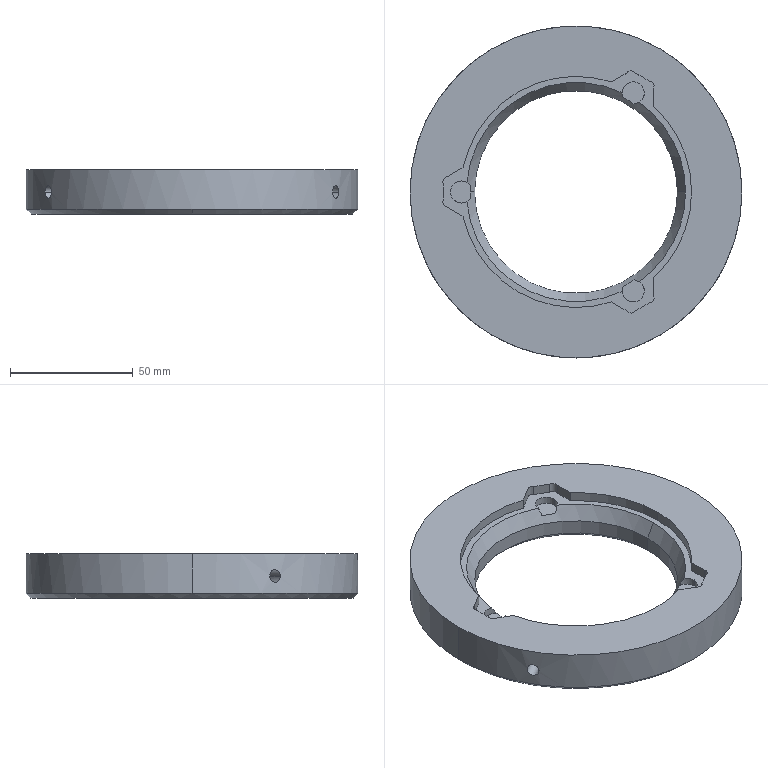Part | STEP file | Hub chuck-Mkt | 1 solid | 254 faces | box 135 x 135 x 18 mm | volume 146789 mm3 | spline 108 | plane 100 | cylinder 36 | cone 10 | commonest cylinder face diameters 4 x8 9 x7 5 x6 10 x4 94 x4 108 x3